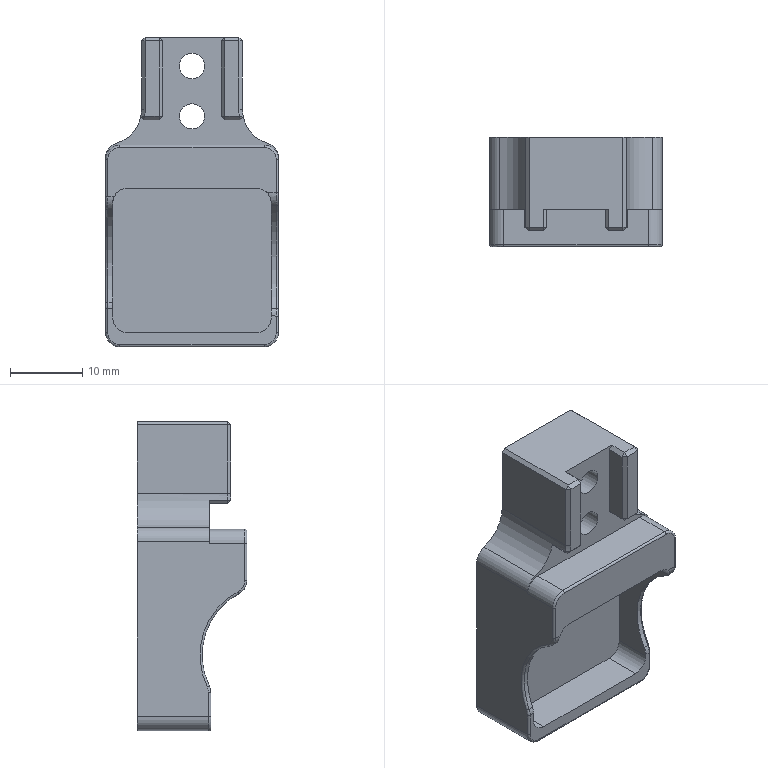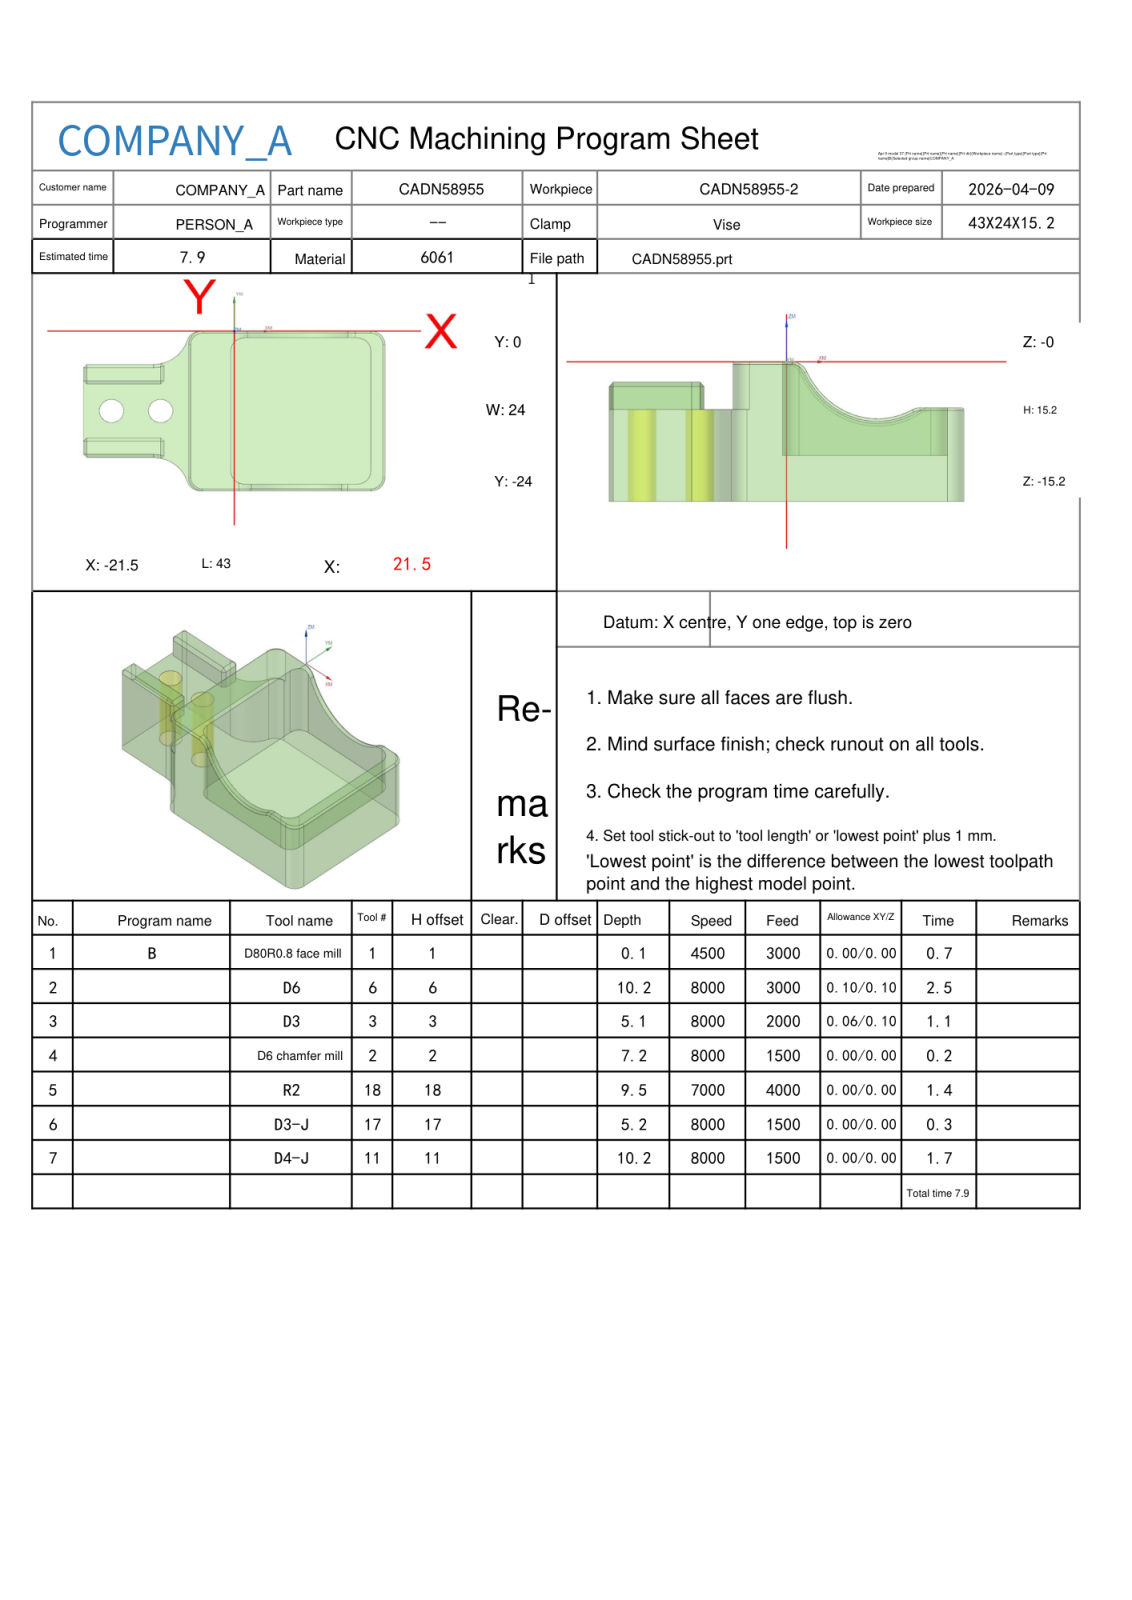NC program | NX | posted by the shop | part box 24 x 15.2 x 43 mm
Lines 2343 to 3233 of 14472:
N3 T03 M06
(D3  D=3. R=0. H=03 ce=0.06 di=0.10)
G00 G90 G54 X-26. Y-12. M03 S8000
G43 H03 Z14.5
M08
Z1.2
G01 Z-.3 F2000.
X-22.97
Y-8.186
X-21.646 Y-9.51
X-9.854
X-8.44 Y-8.096
Y-4.5
X-10.036 Y-3.212
G03 X-8.117 Y-1.009 I-1.464 J3.212
G02 X-5.73 Y1.341 I3.325 J-.991
G03 X-8.06 Y-2. I1.23 J-3.341
G01 Y-22.
G03 X-5.73 Y-25.341 I3.56 J0.0
G02 X-8.117 Y-22.991 I.938 J3.341
G03 X-10.036 Y-20.788 I-3.383 J-1.009
G01 X-8.44 Y-19.5
Y-15.904
X-9.854 Y-14.49
X-21.646
X-22.97 Y-15.814
Y-12.967
G02 X-22.765 Y-12.682 I.3 J0.0
G01 X-20.871 Y-12.05
G03 X-20.696 Y-11.896 I-.095 J.285
G02 X-20.481 Y-11.76 I.216 J-.104
G01 X-10.549
G02 X-10.31 Y-12. I-.001 J-.24
X-10.549 Y-12.24 I-.24 J0.0
G01 X-20.481
G02 X-20.72 Y-12.001 I.001 J.24
G01 Y-11.999
G02 X-20.481 Y-11.76 I.24 J-.001
G01 X-20.358
Z1.2
G00 X-26. Y-12.
Z.9
G01 Z-.6
X-22.97
Y-8.186
X-21.646 Y-9.51
X-9.854
X-8.44 Y-8.096
Y-4.5
X-10.036 Y-3.212
G03 X-8.117 Y-1.009 I-1.464 J3.212
G02 X-5.73 Y1.341 I3.325 J-.991
G03 X-8.06 Y-2. I1.23 J-3.341
G01 Y-22.
G03 X-5.73 Y-25.341 I3.56 J0.0
G02 X-8.117 Y-22.991 I.938 J3.341
G03 X-10.036 Y-20.788 I-3.383 J-1.009
G01 X-8.44 Y-19.5
Y-15.904
X-9.854 Y-14.49
X-21.646
X-22.97 Y-15.814
Y-12.967
G02 X-22.765 Y-12.682 I.3 J0.0
G01 X-20.871 Y-12.05
G03 X-20.696 Y-11.896 I-.095 J.285
G02 X-20.481 Y-11.76 I.216 J-.104
G01 X-10.549
G02 X-10.31 Y-12. I-.001 J-.24
X-10.549 Y-12.24 I-.24 J0.0
G01 X-20.481
G02 X-20.72 Y-12.001 I.001 J.24
G01 Y-11.999
G02 X-20.481 Y-11.76 I.24 J-.001
G01 X-20.358
Z.9
G00 X-26. Y-12.
Z.6
G01 Z-.9
X-22.97
Y-8.186
X-21.646 Y-9.51
X-9.854
X-8.44 Y-8.096
Y-4.5
X-10.036 Y-3.212
G03 X-8.117 Y-1.009 I-1.464 J3.212
G02 X-5.73 Y1.341 I3.325 J-.991
G03 X-8.06 Y-2. I1.23 J-3.341
G01 Y-22.
G03 X-5.73 Y-25.341 I3.56 J0.0
G02 X-8.117 Y-22.991 I.938 J3.341
G03 X-10.036 Y-20.788 I-3.383 J-1.009
G01 X-8.44 Y-19.5
Y-15.904
X-9.854 Y-14.49
X-21.646
X-22.97 Y-15.814
Y-12.967
G02 X-22.765 Y-12.682 I.3 J0.0
G01 X-20.871 Y-12.05
G03 X-20.696 Y-11.896 I-.095 J.285
G02 X-20.481 Y-11.76 I.216 J-.104
G01 X-10.549
G02 X-10.31 Y-12. I-.001 J-.24
X-10.549 Y-12.24 I-.24 J0.0
G01 X-20.481
G02 X-20.72 Y-12.001 I.001 J.24
G01 Y-11.999
G02 X-20.481 Y-11.76 I.24 J-.001
G01 X-20.358
Z.6
G00 X-26. Y-12.
Z.3
G01 Z-1.2
X-22.97
Y-8.186
X-21.646 Y-9.51
X-9.854
X-8.44 Y-8.096
Y-4.5
X-10.036 Y-3.212
G03 X-8.117 Y-1.009 I-1.464 J3.212
G02 X-5.73 Y1.341 I3.325 J-.991
G03 X-8.06 Y-2. I1.23 J-3.341
G01 Y-22.
G03 X-5.73 Y-25.341 I3.56 J0.0
G02 X-8.117 Y-22.991 I.938 J3.341
G03 X-10.036 Y-20.788 I-3.383 J-1.009
G01 X-8.44 Y-19.5
Y-15.904
X-9.854 Y-14.49
X-21.646
X-22.97 Y-15.814
Y-12.967
G02 X-22.765 Y-12.682 I.3 J0.0
G01 X-20.871 Y-12.05
G03 X-20.696 Y-11.896 I-.095 J.285
G02 X-20.481 Y-11.76 I.216 J-.104
G01 X-10.549
G02 X-10.31 Y-12. I-.001 J-.24
X-10.549 Y-12.24 I-.24 J0.0
G01 X-20.481
G02 X-20.72 Y-12.001 I.001 J.24
G01 Y-11.999
G02 X-20.481 Y-11.76 I.24 J-.001
G01 X-20.358
Z.3
G00 X-26. Y-12.
Z0.0
G01 Z-1.5
X-22.97
Y-8.186
X-21.646 Y-9.51
X-9.854
X-8.44 Y-8.096
Y-4.5
X-10.036 Y-3.212
G03 X-8.117 Y-1.009 I-1.464 J3.212
G02 X-5.73 Y1.341 I3.325 J-.991
G03 X-8.06 Y-2. I1.23 J-3.341
G01 Y-22.
G03 X-5.73 Y-25.341 I3.56 J0.0
G02 X-8.117 Y-22.991 I.938 J3.341
G03 X-10.036 Y-20.788 I-3.383 J-1.009
G01 X-8.44 Y-19.5
Y-15.904
X-9.854 Y-14.49
X-21.646
X-22.97 Y-15.814
Y-12.967
G02 X-22.765 Y-12.682 I.3 J0.0
G01 X-20.871 Y-12.05
G03 X-20.696 Y-11.896 I-.095 J.285
G02 X-20.481 Y-11.76 I.216 J-.104
G01 X-10.549
G02 X-10.31 Y-12. I-.001 J-.24
X-10.549 Y-12.24 I-.24 J0.0
G01 X-20.481
G02 X-20.72 Y-12.001 I.001 J.24
G01 Y-11.999
G02 X-20.481 Y-11.76 I.24 J-.001
G01 X-20.358
Z0.0
G00 X-26. Y-12.
Z-.3
G01 Z-1.8
X-22.97
Y-8.186
X-21.646 Y-9.51
X-9.854
X-8.44 Y-8.096
Y-4.5
X-10.036 Y-3.212
G03 X-8.117 Y-1.009 I-1.464 J3.212
G02 X-5.73 Y1.341 I3.325 J-.991
G03 X-8.06 Y-2. I1.23 J-3.341
G01 Y-22.
G03 X-5.73 Y-25.341 I3.56 J0.0
G02 X-8.117 Y-22.991 I.938 J3.341
G03 X-10.036 Y-20.788 I-3.383 J-1.009
G01 X-8.44 Y-19.5
Y-15.904
X-9.854 Y-14.49
X-21.646
X-22.97 Y-15.814
Y-12.967
G02 X-22.765 Y-12.682 I.3 J0.0
G01 X-20.871 Y-12.05
G03 X-20.696 Y-11.896 I-.095 J.285
G02 X-20.481 Y-11.76 I.216 J-.104
G01 X-10.549
G02 X-10.31 Y-12. I-.001 J-.24
X-10.549 Y-12.24 I-.24 J0.0
G01 X-20.481
G02 X-20.72 Y-12.001 I.001 J.24
G01 Y-11.999
G02 X-20.481 Y-11.76 I.24 J-.001
G01 X-20.358
Z-.3
G00 X-26. Y-12.
Z-.6
G01 Z-2.1
X-22.97
Y-8.186
X-21.646 Y-9.51
X-9.854
X-8.44 Y-8.096
Y-4.5
X-10.036 Y-3.212
G03 X-8.117 Y-1.009 I-1.464 J3.212
G02 X-5.73 Y1.341 I3.325 J-.991
G03 X-8.06 Y-2. I1.23 J-3.341
G01 Y-22.
G03 X-5.73 Y-25.341 I3.56 J0.0
G02 X-8.117 Y-22.991 I.938 J3.341
G03 X-10.036 Y-20.788 I-3.383 J-1.009
G01 X-8.44 Y-19.5
Y-15.904
X-9.854 Y-14.49
X-21.646
X-22.97 Y-15.814
Y-12.967
G02 X-22.765 Y-12.682 I.3 J0.0
G01 X-20.871 Y-12.05
G03 X-20.696 Y-11.896 I-.095 J.285
G02 X-20.481 Y-11.76 I.216 J-.104
G01 X-10.549
G02 X-10.31 Y-12. I-.001 J-.24
X-10.549 Y-12.24 I-.24 J0.0
G01 X-20.481
G02 X-20.72 Y-12.001 I.001 J.24
G01 Y-11.999
G02 X-20.481 Y-11.76 I.24 J-.001
G01 X-20.358
Z-.6
G00 X-26. Y-12.
Z-.9
G01 Z-2.4
X-22.97
Y-8.186
X-21.646 Y-9.51
X-9.854
X-8.44 Y-8.096
Y-4.5
X-10.036 Y-3.212
G03 X-8.117 Y-1.009 I-1.464 J3.212
G02 X-5.73 Y1.341 I3.325 J-.991
G03 X-8.06 Y-2. I1.23 J-3.341
G01 Y-22.
G03 X-5.73 Y-25.341 I3.56 J0.0
G02 X-8.117 Y-22.991 I.938 J3.341
G03 X-10.036 Y-20.788 I-3.383 J-1.009
G01 X-8.44 Y-19.5
Y-15.904
X-9.854 Y-14.49
X-21.646
X-22.97 Y-15.814
Y-12.967
G02 X-22.765 Y-12.682 I.3 J0.0
G01 X-20.871 Y-12.05
G03 X-20.696 Y-11.896 I-.095 J.285
G02 X-20.481 Y-11.76 I.216 J-.104
G01 X-10.549
G02 X-10.31 Y-12. I-.001 J-.24
X-10.549 Y-12.24 I-.24 J0.0
G01 X-20.481
G02 X-20.72 Y-12.001 I.001 J.24
G01 Y-11.999
G02 X-20.481 Y-11.76 I.24 J-.001
G01 X-20.358
X-17.369 Y-11.499
X-26.
Z-.9
G00 Y-12.
Z-1.2
G01 Z-2.7
X-22.97
Y-8.186
X-21.646 Y-9.51
X-9.854
X-8.44 Y-8.096
Y-4.5
X-10.036 Y-3.212
G03 X-8.117 Y-1.009 I-1.464 J3.212
G02 X-5.73 Y1.341 I3.325 J-.991
G03 X-8.06 Y-2. I1.23 J-3.341
G01 Y-22.
G03 X-5.73 Y-25.341 I3.56 J0.0
G02 X-8.117 Y-22.991 I.938 J3.341
G03 X-10.036 Y-20.788 I-3.383 J-1.009
G01 X-8.44 Y-19.5
Y-15.904
X-9.854 Y-14.49
X-21.646
X-22.97 Y-15.814
Y-12.967
G02 X-22.765 Y-12.682 I.3 J0.0
G01 X-20.871 Y-12.05
G03 X-20.696 Y-11.896 I-.095 J.285
G02 X-20.481 Y-11.76 I.216 J-.104
G01 X-10.549
G02 X-10.31 Y-12. I-.001 J-.24
X-10.549 Y-12.24 I-.24 J0.0
G01 X-20.481
G02 X-20.72 Y-12.001 I.001 J.24
G01 Y-11.999
G02 X-20.481 Y-11.76 I.24 J-.001
G01 X-20.358
X-17.369 Y-11.499
X-26.
Z-1.2
G00 Y-12.
Z-1.5
G01 Z-3.
X-22.97
Y-8.186
X-21.646 Y-9.51
X-9.854
X-8.44 Y-8.096
Y-4.5
X-10.036 Y-3.212
G03 X-8.117 Y-1.009 I-1.464 J3.212
G02 X-5.73 Y1.341 I3.325 J-.991
G03 X-8.06 Y-2. I1.23 J-3.341
G01 Y-22.
G03 X-5.73 Y-25.341 I3.56 J0.0
G02 X-8.117 Y-22.991 I.938 J3.341
G03 X-10.036 Y-20.788 I-3.383 J-1.009
G01 X-8.44 Y-19.5
Y-15.904
X-9.854 Y-14.49
X-21.646
X-22.97 Y-15.814
Y-12.967
G02 X-22.765 Y-12.682 I.3 J0.0
G01 X-20.871 Y-12.05
G03 X-20.696 Y-11.896 I-.095 J.285
G02 X-20.481 Y-11.76 I.216 J-.104
G01 X-10.549
G02 X-10.31 Y-12. I-.001 J-.24
X-10.549 Y-12.24 I-.24 J0.0
G01 X-20.481
G02 X-20.72 Y-12.001 I.001 J.24
G01 Y-11.999
G02 X-20.481 Y-11.76 I.24 J-.001
G01 X-20.358
X-17.369 Y-11.499
X-26.
Z-1.5
G00 Y-12.
Z-1.8
G01 Z-3.3
X-22.97
Y-8.186
X-21.646 Y-9.51
X-9.854
X-8.44 Y-8.096
Y-4.5
X-10.036 Y-3.212
G03 X-8.117 Y-1.009 I-1.464 J3.212
G02 X-5.73 Y1.341 I3.325 J-.991
G03 X-8.06 Y-2. I1.23 J-3.341
G01 Y-22.
G03 X-5.73 Y-25.341 I3.56 J0.0
G02 X-8.117 Y-22.991 I.938 J3.341
G03 X-10.036 Y-20.788 I-3.383 J-1.009
G01 X-8.44 Y-19.5
Y-15.904
X-9.854 Y-14.49
X-21.646
X-22.97 Y-15.814
Y-12.967
G02 X-22.765 Y-12.682 I.3 J0.0
G01 X-20.871 Y-12.05
G03 X-20.696 Y-11.896 I-.095 J.285
G02 X-20.481 Y-11.76 I.216 J-.104
G01 X-10.549
G02 X-10.31 Y-12. I-.001 J-.24
X-10.549 Y-12.24 I-.24 J0.0
G01 X-20.481
G02 X-20.72 Y-12.001 I.001 J.24
G01 Y-11.999
G02 X-20.481 Y-11.76 I.24 J-.001
G01 X-20.358
X-17.369 Y-11.499
X-26.
Z-1.8
G00 Y-12.
Z-2.1
G01 Z-3.6
X-22.97
Y-8.186
X-21.646 Y-9.51
X-9.854
X-8.44 Y-8.096
Y-4.5
X-10.036 Y-3.212
G03 X-8.117 Y-1.009 I-1.464 J3.212
G02 X-5.73 Y1.341 I3.325 J-.991
G03 X-8.06 Y-2. I1.23 J-3.341
G01 Y-22.
G03 X-5.73 Y-25.341 I3.56 J0.0
G02 X-8.117 Y-22.991 I.938 J3.341
G03 X-10.036 Y-20.788 I-3.383 J-1.009
G01 X-8.44 Y-19.5
Y-15.904
X-9.854 Y-14.49
X-21.646
X-22.97 Y-15.814
Y-12.967
G02 X-22.765 Y-12.682 I.3 J0.0
G01 X-20.871 Y-12.05
G03 X-20.696 Y-11.896 I-.095 J.285
G02 X-20.481 Y-11.76 I.216 J-.104
G01 X-10.549
G02 X-10.31 Y-12. I-.001 J-.24
X-10.549 Y-12.24 I-.24 J0.0
G01 X-20.481
G02 X-20.72 Y-12.001 I.001 J.24
G01 Y-11.999
G02 X-20.481 Y-11.76 I.24 J-.001
G01 X-20.358
X-17.369 Y-11.499
X-26.
Z-2.1
G00 Y-12.
Z-2.4
G01 Z-3.9
X-22.97
Y-8.186
X-21.646 Y-9.51
X-9.854
X-8.44 Y-8.096
Y-4.5
X-10.036 Y-3.212
G03 X-8.117 Y-1.009 I-1.464 J3.212
G02 X-5.73 Y1.341 I3.325 J-.991
G03 X-8.06 Y-2. I1.23 J-3.341
G01 Y-22.
G03 X-5.73 Y-25.341 I3.56 J0.0
G02 X-8.117 Y-22.991 I.938 J3.341
G03 X-10.036 Y-20.788 I-3.383 J-1.009
G01 X-8.44 Y-19.5
Y-15.904
X-9.854 Y-14.49
X-21.646
X-22.97 Y-15.814
Y-12.967
G02 X-22.765 Y-12.682 I.3 J0.0
G01 X-20.871 Y-12.05
G03 X-20.696 Y-11.896 I-.095 J.285
G02 X-20.481 Y-11.76 I.216 J-.104
G01 X-10.549
G02 X-10.31 Y-12. I-.001 J-.24
X-10.549 Y-12.24 I-.24 J0.0
G01 X-20.481
G02 X-20.72 Y-12.001 I.001 J.24
G01 Y-11.999
G02 X-20.481 Y-11.76 I.24 J-.001
G01 X-20.358
X-17.369 Y-11.499
X-26.
Z-2.4
G00 Y-12.
Z-2.7
G01 Z-4.2
X-22.97
Y-8.186
X-21.646 Y-9.51
X-9.854
X-8.44 Y-8.096
Y-4.5
X-10.036 Y-3.212
G03 X-8.117 Y-1.009 I-1.464 J3.212
G02 X-5.73 Y1.341 I3.325 J-.991
G03 X-8.06 Y-2. I1.23 J-3.341
G01 Y-22.
G03 X-5.73 Y-25.341 I3.56 J0.0
G02 X-8.117 Y-22.991 I.938 J3.341
G03 X-10.036 Y-20.788 I-3.383 J-1.009
G01 X-8.44 Y-19.5
Y-15.904
X-9.854 Y-14.49
X-21.646
X-22.97 Y-15.814
Y-12.967
G02 X-22.765 Y-12.682 I.3 J0.0
G01 X-20.871 Y-12.05
G03 X-20.696 Y-11.896 I-.095 J.285
G02 X-20.481 Y-11.76 I.216 J-.104
G01 X-10.549
G02 X-10.31 Y-12. I-.001 J-.24
X-10.549 Y-12.24 I-.24 J0.0
G01 X-20.481
G02 X-20.72 Y-12.001 I.001 J.24
G01 Y-11.999
G02 X-20.481 Y-11.76 I.24 J-.001
G01 X-20.358
X-17.369 Y-11.499
X-26.
Z-2.7
G00 Y-12.
Z-3.
G01 Z-4.5
X-22.97
Y-8.186
X-21.646 Y-9.51
X-9.854
X-8.44 Y-8.096
Y-4.5
X-10.036 Y-3.212
G03 X-8.117 Y-1.009 I-1.464 J3.212
G02 X-5.73 Y1.341 I3.325 J-.991
G03 X-8.06 Y-2. I1.23 J-3.341
G01 Y-22.
G03 X-5.73 Y-25.341 I3.56 J0.0
G02 X-8.117 Y-22.991 I.938 J3.341
G03 X-10.036 Y-20.788 I-3.383 J-1.009
G01 X-8.44 Y-19.5
Y-15.904
X-9.854 Y-14.49
X-21.646
X-22.97 Y-15.814
Y-12.967
G02 X-22.765 Y-12.682 I.3 J0.0
G01 X-20.871 Y-12.05
G03 X-20.696 Y-11.896 I-.095 J.285
G02 X-20.481 Y-11.76 I.216 J-.104
G01 X-10.549
G02 X-10.31 Y-12. I-.001 J-.24
X-10.549 Y-12.24 I-.24 J0.0
G01 X-20.481
G02 X-20.72 Y-12.001 I.001 J.24
G01 Y-11.999
G02 X-20.481 Y-11.76 I.24 J-.001
G01 X-20.358
X-17.369 Y-11.499
X-26.
Z-3.
G00 Y-12.
Z-3.3
G01 Z-4.8
X-22.97
Y-8.186
X-21.646 Y-9.51
X-9.854
X-8.44 Y-8.096
Y-4.5
X-10.036 Y-3.212
G03 X-8.117 Y-1.009 I-1.464 J3.212
G02 X-5.73 Y1.341 I3.325 J-.991
G03 X-8.06 Y-2. I1.23 J-3.341
G01 Y-22.
G03 X-5.73 Y-25.341 I3.56 J0.0
G02 X-8.117 Y-22.991 I.938 J3.341
G03 X-10.036 Y-20.788 I-3.383 J-1.009
G01 X-8.44 Y-19.5
Y-15.904
X-9.854 Y-14.49
X-21.646
X-22.97 Y-15.814
Y-12.967
G02 X-22.765 Y-12.682 I.3 J0.0
G01 X-20.871 Y-12.05
G03 X-20.696 Y-11.896 I-.095 J.285
G02 X-20.481 Y-11.76 I.216 J-.104
G01 X-10.549
G02 X-10.31 Y-12. I-.001 J-.24
X-10.549 Y-12.24 I-.24 J0.0
G01 X-20.481
G02 X-20.72 Y-12.001 I.001 J.24
G01 Y-11.999
G02 X-20.481 Y-11.76 I.24 J-.001
G01 X-20.358
X-17.369 Y-11.499
X-26.
Z-3.3
G00 Y-12.
Z-3.6
G01 Z-5.1
X-22.97
Y-8.186
X-21.646 Y-9.51
X-9.854
X-8.44 Y-8.096
Y-4.5
X-10.036 Y-3.212
G03 X-8.117 Y-1.009 I-1.464 J3.212
G02 X-5.73 Y1.341 I3.325 J-.991
G03 X-8.06 Y-2. I1.23 J-3.341
G01 Y-22.
G03 X-5.73 Y-25.341 I3.56 J0.0
G02 X-8.117 Y-22.991 I.938 J3.341
G03 X-10.036 Y-20.788 I-3.383 J-1.009
G01 X-8.44 Y-19.5
Y-15.904
X-9.854 Y-14.49
X-21.646
X-22.97 Y-15.814
Y-12.967
G02 X-22.765 Y-12.682 I.3 J0.0
G01 X-20.871 Y-12.05
G03 X-20.696 Y-11.896 I-.095 J.285
G02 X-20.481 Y-11.76 I.216 J-.104
G01 X-10.549
G02 X-10.31 Y-12. I-.001 J-.24
X-10.549 Y-12.24 I-.24 J0.0
G01 X-20.481
G02 X-20.72 Y-12.001 I.001 J.24
G01 Y-11.999
G02 X-20.481 Y-11.76 I.24 J-.001
G01 X-20.358
X-17.369 Y-11.499
X-26.
Z-3.6
G00 Z14.5
G91 G28 Z0.0
M05
M09
G91 G28 Z0.0
M01
N4 T02 M06
(D6 chamfer mill D=6. R=0. H=02 ce=0.00 di=0.10)
G00 G90 G54 X-17.5 Y-12. M03 S8000
G43 H02 Z-4.
M08
G98 G81 X-17.5 Y-12. Z19.15 R24.2 F1000.
X-10.5
G80
G00 Z-4.
G00 G90 X-10.5 Y-12. M03 S8000
Z20.
G98 G81 X-10.5 Y-12. Z-7.25 R-2.2 F1000.
X-17.5
G80
G00 Z20.
G00 G90 X1.234 Y-2.114 M03 S6500
Z20.
Z.243
G01 Z-1.199 F1500.
G03 X.899 Y-2.211 I.383 J-1.963
G01 X.847 Y-2.228
X.815 Y-2.272
X.644 Y-2.482
X.537 Y-2.731
X.5 Y-3.
Y-21.
G03 X1.076 Y-21.906 I1. J0.0
G01 X1.121 Y-21.937
X1.175 Y-21.935
X1.23 Y-21.936
G03 X1.523 Y-21.914 I0.0 J2.
G01 Z.222
G00 Z10.
X15.808 Y-21.773
Z-4.853
G01 Z-6.199
G03 X16.094 Y-21.973 I1.286 J1.532
G01 X16.139 Y-22.003
X16.194 Y-22.
X17.5
G03 X18.5 Y-21. I0.0 J1.
G01 Y-3.
G03 X17.5 Y-2. I-1. J0.0
G01 X17.201
X17.147 Y-1.997
X17.101 Y-2.027
G03 X16.815 Y-2.227 I1. J-1.732
G01 Z-4.852
G00 Z10.
X-22.568 Y-13.253
Z-4.327
G01 Z-6.399
X-22.508 Y-13.168
X-22.5 Y-13.138
Y-10.863
X-22.508 Y-10.833
X-22.568 Y-10.747
Z-4.327
G00 Z10.
X-9.837 Y-12.249
Z-2.115
G01 Z-6.399
G03 X-9.762 Y-11.909 I-1.907 J.601
G01 X-9.752 Y-11.855
X-9.776 Y-11.806
G03 X-10.5 Y-11.25 I-.724 J-.194
X-11.25 Y-12. I0.0 J-.75
X-10.5 Y-12.75 I.75 J0.0
X-9.776 Y-12.194 I0.0 J.75
G01 X-9.752 Y-12.145
X-9.762 Y-12.091
G03 X-9.837 Y-11.751 I-1.983 J-.261
G01 Z-2.115
G00 Z1.101
X-16.924 Y-12.412
Z-4.327
G01 Z-6.399
G03 X-16.764 Y-12.103 I-1.687 J1.075
G01 X-16.74 Y-12.054
X-16.75 Y-12.
G03 X-17.5 Y-11.25 I-.75 J0.0
X-18.25 Y-12. I0.0 J-.75
X-17.5 Y-12.75 I.75 J0.0
X-16.776 Y-12.194 I0.0 J.75
G01 X-16.75 Y-12.
X-16.74 Y-11.946
X-16.764 Y-11.897
G03 X-16.924 Y-11.588 I-1.848 J-.765
G01 Z-4.327
G00 Z20.
G00 G90 X1.576 Y-2.479 M03 S6500
Z20.
Z-.256
G01 Z-1.499 F1500.
G03 X1.241 Y-2.575 I.383 J-1.963
G01 X1.189 Y-2.592
X1.157 Y-2.636
X1.072 Y-2.741
X1.018 Y-2.866
X1. Y-3.
Y-21.
X1.035 Y-21.184
X1.136 Y-21.343
X1.288 Y-21.453
X1.33 Y-21.487
X1.385 Y-21.49
G03 X1.59 Y-21.5 I.205 J1.989
G01 X1.733 Y-21.495
Z-.246
G00 Z2.251
X-9.691 Y-19.898
Z-1.968
G01 Z-3.699
X-9.76 Y-19.897
X-9.78 Y-19.903
X-9.814 Y-19.926
X-10.121 Y-20.043
X-10.445 Y-20.091
X-10.773 Y-20.067
X-11.135 Y-20.017
X-11.5 Y-20.
X-15.884
X-21.
G02 X-22.5 Y-18.5 I0.0 J1.5
G01 Y-16.55
G02 X-21. Y-15.05 I1.5 J0.0
G01 X-10.5
X-10.166 Y-15.088
X-9.849 Y-15.199
X-9.778 Y-15.243
X-9.768 Y-15.246
X-9.733 Y-15.245
Z-2.01
G00 Z.051
Y-8.755
Z-2.01
G01 Z-3.699
X-9.768 Y-8.754
X-9.778 Y-8.757
X-9.849 Y-8.801
X-10.166 Y-8.912
X-10.5 Y-8.95
X-15.75
X-21.
G02 X-22.5 Y-7.45 I0.0 J1.5
G01 Y-5.5
G02 X-21. Y-4. I1.5 J0.0
G01 X-11.5
X-11.135 Y-3.983
X-10.773 Y-3.933
X-10.445 Y-3.909
X-10.121 Y-3.957
X-9.814 Y-4.074
X-9.78 Y-4.097
X-9.76 Y-4.103
X-9.691 Y-4.102
Z-1.968
G00 Z10.
X15.808 Y-21.273
Z-5.348
G01 Z-6.499
G03 X16.094 Y-21.473 I1.286 J1.532
G01 X16.139 Y-21.503
X16.194 Y-21.5
X17.5
X17.691 Y-21.462
X17.854 Y-21.354
X17.962 Y-21.191
X18. Y-21.
Y-3.
X17.962 Y-2.809
X17.854 Y-2.646
X17.691 Y-2.538
X17.5 Y-2.5
X17.201
X17.147 Y-2.497
X17.101 Y-2.527
G03 X16.815 Y-2.727 I1. J-1.732
G01 Z-5.348
G00 Z10.
X-23.113 Y-13.65
Z-4.327
G01 Z-6.699
X-23.052 Y-13.587
X-23.013 Y-13.507
X-22.994 Y-13.486
X-23. Y-13.457
Y-10.543
X-22.994 Y-10.514
X-23.013 Y-10.493
X-23.052 Y-10.413
X-23.113 Y-10.35
Z-4.327
G00 Z10.
X-10.31 Y-12.216
Z-2.127
G01 Z-6.699
X-10.267 Y-12.138
X-10.25 Y-12.052
X-10.237 Y-12.026
X-10.25 Y-12.
X-10.283 Y-11.875
X-10.375 Y-11.783
X-10.5 Y-11.75
X-10.625 Y-11.783
X-10.717 Y-11.875
X-10.75 Y-12.
X-10.717 Y-12.125
X-10.625 Y-12.217
X-10.5 Y-12.25
X-10.375 Y-12.217
X-10.283 Y-12.125
X-10.25 Y-12.
X-10.237 Y-11.974
X-10.25 Y-11.948
X-10.267 Y-11.862
X-10.31 Y-11.784
Z-2.127
G00 Z.801
X-17.31 Y-12.216
Z-4.472
G01 Z-6.699
X-17.267 Y-12.138
X-17.25 Y-12.052
X-17.237 Y-12.026
X-17.25 Y-12.
X-17.283 Y-11.875
X-17.375 Y-11.783
X-17.5 Y-11.75
X-17.625 Y-11.783
X-17.717 Y-11.875
X-17.75 Y-12.
X-17.717 Y-12.125
X-17.625 Y-12.217
X-17.5 Y-12.25
X-17.375 Y-12.217
X-17.283 Y-12.125
X-17.25 Y-12.
X-17.237 Y-11.974
X-17.25 Y-11.948
X-17.267 Y-11.862
X-17.31 Y-11.784
Z-4.472
G00 Z20.
G91 G28 Z0.0
M05
M09
G91 G28 Z0.0
M01